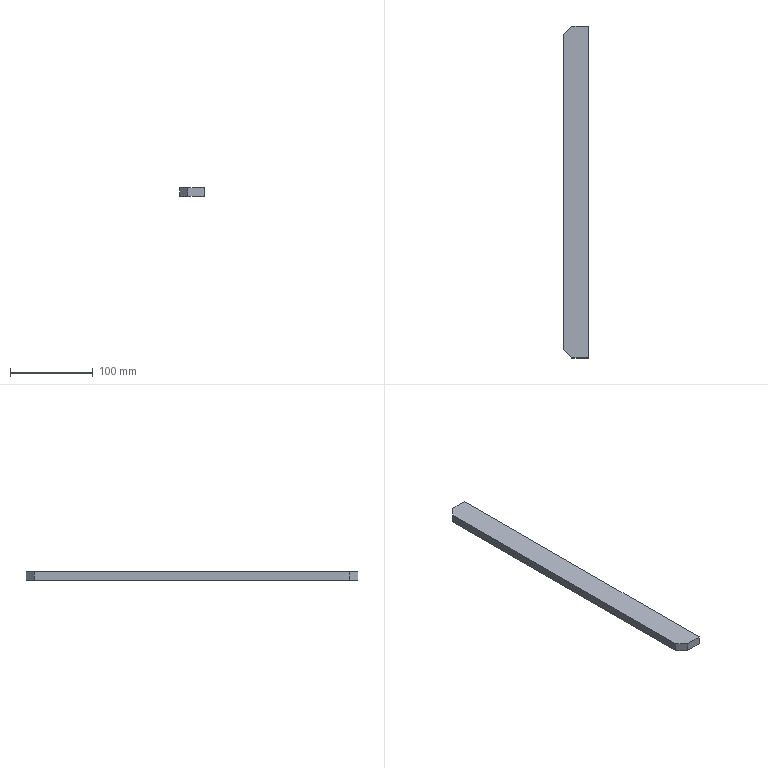Part | STEP file | DSJIN2 | 1 solid | 28 faces | box 30 x 400 x 10 mm | volume 118112 mm3 | cylinder 10 | cone 10 | plane 8 | commonest cylinder face diameters 4.2 x10
STEP:
#1=CARTESIAN_POINT('',(2.6,100.,6.1));
#2=VERTEX_POINT('',#1);
#3=CARTESIAN_POINT('',(2.6,100.,1.9));
#4=VERTEX_POINT('',#3);
#5=CARTESIAN_POINT('',(2.6,100.,4.));
#6=DIRECTION('',(1.,0.,0.));
#7=DIRECTION('',(0.,0.,-1.));
#8=AXIS2_PLACEMENT_3D('',#5,#6,#7);
#9=CIRCLE('',#8,2.1);
#10=EDGE_CURVE('',#2,#4,#9,.T.);
#11=ORIENTED_EDGE('',*,*,#10,.F.);
#12=CARTESIAN_POINT('',(15.,100.,6.1));
#13=VERTEX_POINT('',#12);
#14=CARTESIAN_POINT('',(15.,100.,6.1));
#15=DIRECTION('',(1.,0.,0.));
#16=VECTOR('',#15,1000.);
#17=LINE('',#14,#16);
#18=EDGE_CURVE('',#2,#13,#17,.T.);
#19=ORIENTED_EDGE('',*,*,#18,.T.);
#20=CARTESIAN_POINT('',(15.,100.,1.9));
#21=VERTEX_POINT('',#20);
#22=CARTESIAN_POINT('',(15.,100.,4.));
#23=DIRECTION('',(1.,0.,0.));
#24=DIRECTION('',(0.,0.,-1.));
#25=AXIS2_PLACEMENT_3D('',#22,#23,#24);
#26=CIRCLE('',#25,2.1);
#27=EDGE_CURVE('',#13,#21,#26,.T.);
#28=ORIENTED_EDGE('',*,*,#27,.T.);
#29=CARTESIAN_POINT('',(15.,100.,1.9));
#30=DIRECTION('',(1.,0.,0.));
#31=VECTOR('',#30,1000.);
#32=LINE('',#29,#31);
#33=EDGE_CURVE('',#4,#21,#32,.T.);
#34=ORIENTED_EDGE('',*,*,#33,.F.);
#35=EDGE_LOOP('',(#11,#19,#28,#34));
#36=FACE_OUTER_BOUND('',#35,.T.);
#37=CARTESIAN_POINT('',(15.,100.,4.));
#38=DIRECTION('',(1.,0.,0.));
#39=DIRECTION('',(0.,0.,-1.));
#40=AXIS2_PLACEMENT_3D('',#37,#38,#39);
#41=CYLINDRICAL_SURFACE('',#40,2.1);
#42=ADVANCED_FACE('',(#36),#41,.F.);
#43=CARTESIAN_POINT('',(1.338,100.,4.));
#44=VERTEX_POINT('',#43);
#45=CARTESIAN_POINT('',(2.6,100.,1.9));
#46=DIRECTION('',(0.515,0.,-0.8572));
#47=VECTOR('',#46,1000.);
#48=LINE('',#45,#47);
#49=EDGE_CURVE('',#44,#4,#48,.T.);
#50=ORIENTED_EDGE('',*,*,#49,.F.);
#51=CARTESIAN_POINT('',(2.6,100.,6.1));
#52=DIRECTION('',(0.515,0.,0.8572));
#53=VECTOR('',#52,1000.);
#54=LINE('',#51,#53);
#55=EDGE_CURVE('',#44,#2,#54,.T.);
#56=ORIENTED_EDGE('',*,*,#55,.T.);
#57=ORIENTED_EDGE('',*,*,#10,.T.);
#58=EDGE_LOOP('',(#50,#56,#57));
#59=FACE_OUTER_BOUND('',#58,.T.);
#60=CARTESIAN_POINT('',(2.6,100.,4.));
#61=DIRECTION('',(1.,0.,0.));
#62=DIRECTION('',(0.,0.,-1.));
#63=AXIS2_PLACEMENT_3D('',#60,#61,#62);
#64=CONICAL_SURFACE('',#63,2.1,1.03);
#65=ADVANCED_FACE('',(#59),#64,.F.);
#66=CARTESIAN_POINT('',(2.6,0.,6.1));
#67=VERTEX_POINT('',#66);
#68=CARTESIAN_POINT('',(2.6,0.,1.9));
#69=VERTEX_POINT('',#68);
#70=CARTESIAN_POINT('',(2.6,0.,4.));
#71=DIRECTION('',(1.,0.,0.));
#72=DIRECTION('',(0.,0.,-1.));
#73=AXIS2_PLACEMENT_3D('',#70,#71,#72);
#74=CIRCLE('',#73,2.1);
#75=EDGE_CURVE('',#67,#69,#74,.T.);
#76=ORIENTED_EDGE('',*,*,#75,.F.);
#77=CARTESIAN_POINT('',(15.,0.,6.1));
#78=VERTEX_POINT('',#77);
#79=CARTESIAN_POINT('',(15.,0.,6.1));
#80=DIRECTION('',(1.,0.,0.));
#81=VECTOR('',#80,1000.);
#82=LINE('',#79,#81);
#83=EDGE_CURVE('',#67,#78,#82,.T.);
#84=ORIENTED_EDGE('',*,*,#83,.T.);
#85=CARTESIAN_POINT('',(15.,0.,1.9));
#86=VERTEX_POINT('',#85);
#87=CARTESIAN_POINT('',(15.,0.,4.));
#88=DIRECTION('',(1.,0.,0.));
#89=DIRECTION('',(0.,0.,-1.));
#90=AXIS2_PLACEMENT_3D('',#87,#88,#89);
#91=CIRCLE('',#90,2.1);
#92=EDGE_CURVE('',#78,#86,#91,.T.);
#93=ORIENTED_EDGE('',*,*,#92,.T.);
#94=CARTESIAN_POINT('',(15.,0.,1.9));
#95=DIRECTION('',(1.,0.,0.));
#96=VECTOR('',#95,1000.);
#97=LINE('',#94,#96);
#98=EDGE_CURVE('',#69,#86,#97,.T.);
#99=ORIENTED_EDGE('',*,*,#98,.F.);
#100=EDGE_LOOP('',(#76,#84,#93,#99));
#101=FACE_OUTER_BOUND('',#100,.T.);
#102=CARTESIAN_POINT('',(15.,0.,4.));
#103=DIRECTION('',(1.,0.,0.));
#104=DIRECTION('',(0.,0.,-1.));
#105=AXIS2_PLACEMENT_3D('',#102,#103,#104);
#106=CYLINDRICAL_SURFACE('',#105,2.1);
#107=ADVANCED_FACE('',(#101),#106,.F.);
#108=CARTESIAN_POINT('',(1.338,0.,4.));
#109=VERTEX_POINT('',#108);
#110=CARTESIAN_POINT('',(2.6,0.,1.9));
#111=DIRECTION('',(0.515,0.,-0.8572));
#112=VECTOR('',#111,1000.);
#113=LINE('',#110,#112);
#114=EDGE_CURVE('',#109,#69,#113,.T.);
#115=ORIENTED_EDGE('',*,*,#114,.F.);
#116=CARTESIAN_POINT('',(2.6,0.,6.1));
#117=DIRECTION('',(0.515,0.,0.8572));
#118=VECTOR('',#117,1000.);
#119=LINE('',#116,#118);
#120=EDGE_CURVE('',#109,#67,#119,.T.);
#121=ORIENTED_EDGE('',*,*,#120,.T.);
#122=ORIENTED_EDGE('',*,*,#75,.T.);
#123=EDGE_LOOP('',(#115,#121,#122));
#124=FACE_OUTER_BOUND('',#123,.T.);
#125=CARTESIAN_POINT('',(2.6,0.,4.));
#126=DIRECTION('',(1.,0.,0.));
#127=DIRECTION('',(0.,0.,-1.));
#128=AXIS2_PLACEMENT_3D('',#125,#126,#127);
#129=CONICAL_SURFACE('',#128,2.1,1.03);
#130=ADVANCED_FACE('',(#124),#129,.F.);
#131=CARTESIAN_POINT('',(2.6,-100.,6.1));
#132=VERTEX_POINT('',#131);
#133=CARTESIAN_POINT('',(2.6,-100.,1.9));
#134=VERTEX_POINT('',#133);
#135=CARTESIAN_POINT('',(2.6,-100.,4.));
#136=DIRECTION('',(1.,0.,0.));
#137=DIRECTION('',(0.,0.,-1.));
#138=AXIS2_PLACEMENT_3D('',#135,#136,#137);
#139=CIRCLE('',#138,2.1);
#140=EDGE_CURVE('',#132,#134,#139,.T.);
#141=ORIENTED_EDGE('',*,*,#140,.F.);
#142=CARTESIAN_POINT('',(15.,-100.,6.1));
#143=VERTEX_POINT('',#142);
#144=CARTESIAN_POINT('',(15.,-100.,6.1));
#145=DIRECTION('',(1.,0.,0.));
#146=VECTOR('',#145,1000.);
#147=LINE('',#144,#146);
#148=EDGE_CURVE('',#132,#143,#147,.T.);
#149=ORIENTED_EDGE('',*,*,#148,.T.);
#150=CARTESIAN_POINT('',(15.,-100.,1.9));
#151=VERTEX_POINT('',#150);
#152=CARTESIAN_POINT('',(15.,-100.,4.));
#153=DIRECTION('',(1.,0.,0.));
#154=DIRECTION('',(0.,0.,-1.));
#155=AXIS2_PLACEMENT_3D('',#152,#153,#154);
#156=CIRCLE('',#155,2.1);
#157=EDGE_CURVE('',#143,#151,#156,.T.);
#158=ORIENTED_EDGE('',*,*,#157,.T.);
#159=CARTESIAN_POINT('',(15.,-100.,1.9));
#160=DIRECTION('',(1.,0.,0.));
#161=VECTOR('',#160,1000.);
#162=LINE('',#159,#161);
#163=EDGE_CURVE('',#134,#151,#162,.T.);
#164=ORIENTED_EDGE('',*,*,#163,.F.);
#165=EDGE_LOOP('',(#141,#149,#158,#164));
#166=FACE_OUTER_BOUND('',#165,.T.);
#167=CARTESIAN_POINT('',(15.,-100.,4.));
#168=DIRECTION('',(1.,0.,0.));
#169=DIRECTION('',(0.,0.,-1.));
#170=AXIS2_PLACEMENT_3D('',#167,#168,#169);
#171=CYLINDRICAL_SURFACE('',#170,2.1);
#172=ADVANCED_FACE('',(#166),#171,.F.);
#173=CARTESIAN_POINT('',(1.338,-100.,4.));
#174=VERTEX_POINT('',#173);
#175=CARTESIAN_POINT('',(2.6,-100.,1.9));
#176=DIRECTION('',(0.515,0.,-0.8572));
#177=VECTOR('',#176,1000.);
#178=LINE('',#175,#177);
#179=EDGE_CURVE('',#174,#134,#178,.T.);
#180=ORIENTED_EDGE('',*,*,#179,.F.);
#181=CARTESIAN_POINT('',(2.6,-100.,6.1));
#182=DIRECTION('',(0.515,0.,0.8572));
#183=VECTOR('',#182,1000.);
#184=LINE('',#181,#183);
#185=EDGE_CURVE('',#174,#132,#184,.T.);
#186=ORIENTED_EDGE('',*,*,#185,.T.);
#187=ORIENTED_EDGE('',*,*,#140,.T.);
#188=EDGE_LOOP('',(#180,#186,#187));
#189=FACE_OUTER_BOUND('',#188,.T.);
#190=CARTESIAN_POINT('',(2.6,-100.,4.));
#191=DIRECTION('',(1.,0.,0.));
#192=DIRECTION('',(0.,0.,-1.));
#193=AXIS2_PLACEMENT_3D('',#190,#191,#192);
#194=CONICAL_SURFACE('',#193,2.1,1.03);
#195=ADVANCED_FACE('',(#189),#194,.F.);
#196=CARTESIAN_POINT('',(2.6,190.,6.1));
#197=VERTEX_POINT('',#196);
#198=CARTESIAN_POINT('',(2.6,190.,1.9));
#199=VERTEX_POINT('',#198);
#200=CARTESIAN_POINT('',(2.6,190.,4.));
#201=DIRECTION('',(1.,0.,0.));
#202=DIRECTION('',(0.,0.,-1.));
#203=AXIS2_PLACEMENT_3D('',#200,#201,#202);
#204=CIRCLE('',#203,2.1);
#205=EDGE_CURVE('',#197,#199,#204,.T.);
#206=ORIENTED_EDGE('',*,*,#205,.F.);
#207=CARTESIAN_POINT('',(15.,190.,6.1));
#208=VERTEX_POINT('',#207);
#209=CARTESIAN_POINT('',(15.,190.,6.1));
#210=DIRECTION('',(1.,0.,0.));
#211=VECTOR('',#210,1000.);
#212=LINE('',#209,#211);
#213=EDGE_CURVE('',#197,#208,#212,.T.);
#214=ORIENTED_EDGE('',*,*,#213,.T.);
#215=CARTESIAN_POINT('',(15.,190.,1.9));
#216=VERTEX_POINT('',#215);
#217=CARTESIAN_POINT('',(15.,190.,4.));
#218=DIRECTION('',(1.,0.,0.));
#219=DIRECTION('',(0.,0.,-1.));
#220=AXIS2_PLACEMENT_3D('',#217,#218,#219);
#221=CIRCLE('',#220,2.1);
#222=EDGE_CURVE('',#208,#216,#221,.T.);
#223=ORIENTED_EDGE('',*,*,#222,.T.);
#224=CARTESIAN_POINT('',(15.,190.,1.9));
#225=DIRECTION('',(1.,0.,0.));
#226=VECTOR('',#225,1000.);
#227=LINE('',#224,#226);
#228=EDGE_CURVE('',#199,#216,#227,.T.);
#229=ORIENTED_EDGE('',*,*,#228,.F.);
#230=EDGE_LOOP('',(#206,#214,#223,#229));
#231=FACE_OUTER_BOUND('',#230,.T.);
#232=CARTESIAN_POINT('',(15.,190.,4.));
#233=DIRECTION('',(1.,0.,0.));
#234=DIRECTION('',(0.,0.,-1.));
#235=AXIS2_PLACEMENT_3D('',#232,#233,#234);
#236=CYLINDRICAL_SURFACE('',#235,2.1);
#237=ADVANCED_FACE('',(#231),#236,.F.);
#238=CARTESIAN_POINT('',(1.338,190.,4.));
#239=VERTEX_POINT('',#238);
#240=CARTESIAN_POINT('',(2.6,190.,1.9));
#241=DIRECTION('',(0.515,0.,-0.8572));
#242=VECTOR('',#241,1000.);
#243=LINE('',#240,#242);
#244=EDGE_CURVE('',#239,#199,#243,.T.);
#245=ORIENTED_EDGE('',*,*,#244,.F.);
#246=CARTESIAN_POINT('',(2.6,190.,6.1));
#247=DIRECTION('',(0.515,0.,0.8572));
#248=VECTOR('',#247,1000.);
#249=LINE('',#246,#248);
#250=EDGE_CURVE('',#239,#197,#249,.T.);
#251=ORIENTED_EDGE('',*,*,#250,.T.);
#252=ORIENTED_EDGE('',*,*,#205,.T.);
#253=EDGE_LOOP('',(#245,#251,#252));
#254=FACE_OUTER_BOUND('',#253,.T.);
#255=CARTESIAN_POINT('',(2.6,190.,4.));
#256=DIRECTION('',(1.,0.,0.));
#257=DIRECTION('',(0.,0.,-1.));
#258=AXIS2_PLACEMENT_3D('',#255,#256,#257);
#259=CONICAL_SURFACE('',#258,2.1,1.03);
#260=ADVANCED_FACE('',(#254),#259,.F.);
#261=CARTESIAN_POINT('',(2.6,-190.,6.1));
#262=VERTEX_POINT('',#261);
#263=CARTESIAN_POINT('',(2.6,-190.,1.9));
#264=VERTEX_POINT('',#263);
#265=CARTESIAN_POINT('',(2.6,-190.,4.));
#266=DIRECTION('',(1.,0.,0.));
#267=DIRECTION('',(0.,0.,-1.));
#268=AXIS2_PLACEMENT_3D('',#265,#266,#267);
#269=CIRCLE('',#268,2.1);
#270=EDGE_CURVE('',#262,#264,#269,.T.);
#271=ORIENTED_EDGE('',*,*,#270,.F.);
#272=CARTESIAN_POINT('',(15.,-190.,6.1));
#273=VERTEX_POINT('',#272);
#274=CARTESIAN_POINT('',(15.,-190.,6.1));
#275=DIRECTION('',(1.,0.,0.));
#276=VECTOR('',#275,1000.);
#277=LINE('',#274,#276);
#278=EDGE_CURVE('',#262,#273,#277,.T.);
#279=ORIENTED_EDGE('',*,*,#278,.T.);
#280=CARTESIAN_POINT('',(15.,-190.,1.9));
#281=VERTEX_POINT('',#280);
#282=CARTESIAN_POINT('',(15.,-190.,4.));
#283=DIRECTION('',(1.,0.,0.));
#284=DIRECTION('',(0.,0.,-1.));
#285=AXIS2_PLACEMENT_3D('',#282,#283,#284);
#286=CIRCLE('',#285,2.1);
#287=EDGE_CURVE('',#273,#281,#286,.T.);
#288=ORIENTED_EDGE('',*,*,#287,.T.);
#289=CARTESIAN_POINT('',(15.,-190.,1.9));
#290=DIRECTION('',(1.,0.,0.));
#291=VECTOR('',#290,1000.);
#292=LINE('',#289,#291);
#293=EDGE_CURVE('',#264,#281,#292,.T.);
#294=ORIENTED_EDGE('',*,*,#293,.F.);
#295=EDGE_LOOP('',(#271,#279,#288,#294));
#296=FACE_OUTER_BOUND('',#295,.T.);
#297=CARTESIAN_POINT('',(15.,-190.,4.));
#298=DIRECTION('',(1.,0.,0.));
#299=DIRECTION('',(0.,0.,-1.));
#300=AXIS2_PLACEMENT_3D('',#297,#298,#299);
#301=CYLINDRICAL_SURFACE('',#300,2.1);
#302=ADVANCED_FACE('',(#296),#301,.F.);
#303=CARTESIAN_POINT('',(1.338,-190.,4.));
#304=VERTEX_POINT('',#303);
#305=CARTESIAN_POINT('',(2.6,-190.,1.9));
#306=DIRECTION('',(0.515,0.,-0.8572));
#307=VECTOR('',#306,1000.);
#308=LINE('',#305,#307);
#309=EDGE_CURVE('',#304,#264,#308,.T.);
#310=ORIENTED_EDGE('',*,*,#309,.F.);
#311=CARTESIAN_POINT('',(2.6,-190.,6.1));
#312=DIRECTION('',(0.515,0.,0.8572));
#313=VECTOR('',#312,1000.);
#314=LINE('',#311,#313);
#315=EDGE_CURVE('',#304,#262,#314,.T.);
#316=ORIENTED_EDGE('',*,*,#315,.T.);
#317=ORIENTED_EDGE('',*,*,#270,.T.);
#318=EDGE_LOOP('',(#310,#316,#317));
#319=FACE_OUTER_BOUND('',#318,.T.);
#320=CARTESIAN_POINT('',(2.6,-190.,4.));
#321=DIRECTION('',(1.,0.,0.));
#322=DIRECTION('',(0.,0.,-1.));
#323=AXIS2_PLACEMENT_3D('',#320,#321,#322);
#324=CONICAL_SURFACE('',#323,2.1,1.03);
#325=ADVANCED_FACE('',(#319),#324,.F.);
#326=CARTESIAN_POINT('',(15.,100.,4.));
#327=DIRECTION('',(1.,0.,0.));
#328=DIRECTION('',(0.,0.,-1.));
#329=AXIS2_PLACEMENT_3D('',#326,#327,#328);
#330=CIRCLE('',#329,2.1);
#331=EDGE_CURVE('',#21,#13,#330,.T.);
#332=ORIENTED_EDGE('',*,*,#331,.F.);
#333=ORIENTED_EDGE('',*,*,#27,.F.);
#334=EDGE_LOOP('',(#332,#333));
#335=FACE_BOUND('',#334,.T.);
#336=CARTESIAN_POINT('',(15.,0.,4.));
#337=DIRECTION('',(1.,0.,0.));
#338=DIRECTION('',(0.,0.,-1.));
#339=AXIS2_PLACEMENT_3D('',#336,#337,#338);
#340=CIRCLE('',#339,2.1);
#341=EDGE_CURVE('',#86,#78,#340,.T.);
#342=ORIENTED_EDGE('',*,*,#341,.F.);
#343=ORIENTED_EDGE('',*,*,#92,.F.);
#344=EDGE_LOOP('',(#342,#343));
#345=FACE_BOUND('',#344,.T.);
#346=CARTESIAN_POINT('',(15.,-100.,4.));
#347=DIRECTION('',(1.,0.,0.));
#348=DIRECTION('',(0.,0.,-1.));
#349=AXIS2_PLACEMENT_3D('',#346,#347,#348);
#350=CIRCLE('',#349,2.1);
#351=EDGE_CURVE('',#151,#143,#350,.T.);
#352=ORIENTED_EDGE('',*,*,#351,.F.);
#353=ORIENTED_EDGE('',*,*,#157,.F.);
#354=EDGE_LOOP('',(#352,#353));
#355=FACE_BOUND('',#354,.T.);
#356=CARTESIAN_POINT('',(15.,190.,4.));
#357=DIRECTION('',(1.,0.,0.));
#358=DIRECTION('',(0.,0.,-1.));
#359=AXIS2_PLACEMENT_3D('',#356,#357,#358);
#360=CIRCLE('',#359,2.1);
#361=EDGE_CURVE('',#216,#208,#360,.T.);
#362=ORIENTED_EDGE('',*,*,#361,.F.);
#363=ORIENTED_EDGE('',*,*,#222,.F.);
#364=EDGE_LOOP('',(#362,#363));
#365=FACE_BOUND('',#364,.T.);
#366=CARTESIAN_POINT('',(15.,-190.,4.));
#367=DIRECTION('',(1.,0.,0.));
#368=DIRECTION('',(0.,0.,-1.));
#369=AXIS2_PLACEMENT_3D('',#366,#367,#368);
#370=CIRCLE('',#369,2.1);
#371=EDGE_CURVE('',#281,#273,#370,.T.);
#372=ORIENTED_EDGE('',*,*,#371,.F.);
#373=ORIENTED_EDGE('',*,*,#287,.F.);
#374=EDGE_LOOP('',(#372,#373));
#375=FACE_BOUND('',#374,.T.);
#376=CARTESIAN_POINT('',(15.,-200.,0.));
#377=VERTEX_POINT('',#376);
#378=CARTESIAN_POINT('',(15.,200.,0.));
#379=VERTEX_POINT('',#378);
#380=CARTESIAN_POINT('',(15.,-200.,0.));
#381=DIRECTION('',(0.,1.,0.));
#382=VECTOR('',#381,1000.);
#383=LINE('',#380,#382);
#384=EDGE_CURVE('',#377,#379,#383,.T.);
#385=ORIENTED_EDGE('',*,*,#384,.T.);
#386=CARTESIAN_POINT('',(15.,200.,10.));
#387=VERTEX_POINT('',#386);
#388=CARTESIAN_POINT('',(15.,200.,10.));
#389=DIRECTION('',(0.,0.,-1.));
#390=VECTOR('',#389,1000.);
#391=LINE('',#388,#390);
#392=EDGE_CURVE('',#387,#379,#391,.T.);
#393=ORIENTED_EDGE('',*,*,#392,.F.);
#394=CARTESIAN_POINT('',(15.,-200.,10.));
#395=VERTEX_POINT('',#394);
#396=CARTESIAN_POINT('',(15.,-200.,10.));
#397=DIRECTION('',(0.,1.,0.));
#398=VECTOR('',#397,1000.);
#399=LINE('',#396,#398);
#400=EDGE_CURVE('',#395,#387,#399,.T.);
#401=ORIENTED_EDGE('',*,*,#400,.F.);
#402=CARTESIAN_POINT('',(15.,-200.,10.));
#403=DIRECTION('',(0.,0.,-1.));
#404=VECTOR('',#403,1000.);
#405=LINE('',#402,#404);
#406=EDGE_CURVE('',#395,#377,#405,.T.);
#407=ORIENTED_EDGE('',*,*,#406,.T.);
#408=EDGE_LOOP('',(#385,#393,#401,#407));
#409=FACE_OUTER_BOUND('',#408,.T.);
#410=CARTESIAN_POINT('',(15.,-200.,10.));
#411=DIRECTION('',(-1.,0.,0.));
#412=DIRECTION('',(0.,0.,1.));
#413=AXIS2_PLACEMENT_3D('',#410,#411,#412);
#414=PLANE('',#413);
#415=ADVANCED_FACE('',(#335,#345,#355,#365,#375,#409),#414,.F.);
#416=CARTESIAN_POINT('',(-5.,200.,0.));
#417=VERTEX_POINT('',#416);
#418=CARTESIAN_POINT('',(-15.,200.,0.));
#419=DIRECTION('',(-1.,0.,0.));
#420=VECTOR('',#419,1000.);
#421=LINE('',#418,#420);
#422=EDGE_CURVE('',#379,#417,#421,.T.);
#423=ORIENTED_EDGE('',*,*,#422,.T.);
#424=CARTESIAN_POINT('',(-5.,200.,10.));
#425=VERTEX_POINT('',#424);
#426=CARTESIAN_POINT('',(-5.,200.,10.));
#427=DIRECTION('',(0.,0.,1.));
#428=VECTOR('',#427,1000.);
#429=LINE('',#426,#428);
#430=EDGE_CURVE('',#417,#425,#429,.T.);
#431=ORIENTED_EDGE('',*,*,#430,.T.);
#432=CARTESIAN_POINT('',(-15.,200.,10.));
#433=DIRECTION('',(-1.,0.,0.));
#434=VECTOR('',#433,1000.);
#435=LINE('',#432,#434);
#436=EDGE_CURVE('',#387,#425,#435,.T.);
#437=ORIENTED_EDGE('',*,*,#436,.F.);
#438=ORIENTED_EDGE('',*,*,#392,.T.);
#439=EDGE_LOOP('',(#423,#431,#437,#438));
#440=FACE_OUTER_BOUND('',#439,.T.);
#441=CARTESIAN_POINT('',(-15.,200.,10.));
#442=DIRECTION('',(0.,-1.,0.));
#443=DIRECTION('',(0.,0.,-1.));
#444=AXIS2_PLACEMENT_3D('',#441,#442,#443);
#445=PLANE('',#444);
#446=ADVANCED_FACE('',(#440),#445,.F.);
#447=CARTESIAN_POINT('',(-15.,190.,10.));
#448=VERTEX_POINT('',#447);
#449=CARTESIAN_POINT('',(-15.,-190.,10.));
#450=VERTEX_POINT('',#449);
#451=CARTESIAN_POINT('',(-15.,-200.,10.));
#452=DIRECTION('',(0.,-1.,0.));
#453=VECTOR('',#452,1000.);
#454=LINE('',#451,#453);
#455=EDGE_CURVE('',#448,#450,#454,.T.);
#456=ORIENTED_EDGE('',*,*,#455,.F.);
#457=CARTESIAN_POINT('',(-15.,190.,0.));
#458=VERTEX_POINT('',#457);
#459=CARTESIAN_POINT('',(-15.,190.,10.));
#460=DIRECTION('',(0.,0.,-1.));
#461=VECTOR('',#460,1000.);
#462=LINE('',#459,#461);
#463=EDGE_CURVE('',#448,#458,#462,.T.);
#464=ORIENTED_EDGE('',*,*,#463,.T.);
#465=CARTESIAN_POINT('',(-15.,-190.,0.));
#466=VERTEX_POINT('',#465);
#467=CARTESIAN_POINT('',(-15.,-200.,0.));
#468=DIRECTION('',(0.,-1.,0.));
#469=VECTOR('',#468,1000.);
#470=LINE('',#467,#469);
#471=EDGE_CURVE('',#458,#466,#470,.T.);
#472=ORIENTED_EDGE('',*,*,#471,.T.);
#473=CARTESIAN_POINT('',(-15.,-190.,10.));
#474=DIRECTION('',(0.,0.,1.));
#475=VECTOR('',#474,1000.);
#476=LINE('',#473,#475);
#477=EDGE_CURVE('',#466,#450,#476,.T.);
#478=ORIENTED_EDGE('',*,*,#477,.T.);
#479=EDGE_LOOP('',(#456,#464,#472,#478));
#480=FACE_OUTER_BOUND('',#479,.T.);
#481=CARTESIAN_POINT('',(-15.,-200.,10.));
#482=DIRECTION('',(1.,0.,0.));
#483=DIRECTION('',(0.,0.,-1.));
#484=AXIS2_PLACEMENT_3D('',#481,#482,#483);
#485=PLANE('',#484);
#486=ADVANCED_FACE('',(#480),#485,.F.);
#487=CARTESIAN_POINT('',(-5.,-200.,10.));
#488=VERTEX_POINT('',#487);
#489=CARTESIAN_POINT('',(-15.,-200.,10.));
#490=DIRECTION('',(1.,0.,0.));
#491=VECTOR('',#490,1000.);
#492=LINE('',#489,#491);
#493=EDGE_CURVE('',#488,#395,#492,.T.);
#494=ORIENTED_EDGE('',*,*,#493,.F.);
#495=CARTESIAN_POINT('',(-5.,-200.,0.));
#496=VERTEX_POINT('',#495);
#497=CARTESIAN_POINT('',(-5.,-200.,10.));
#498=DIRECTION('',(0.,0.,-1.));
#499=VECTOR('',#498,1000.);
#500=LINE('',#497,#499);
#501=EDGE_CURVE('',#488,#496,#500,.T.);
#502=ORIENTED_EDGE('',*,*,#501,.T.);
#503=CARTESIAN_POINT('',(-15.,-200.,0.));
#504=DIRECTION('',(1.,0.,0.));
#505=VECTOR('',#504,1000.);
#506=LINE('',#503,#505);
#507=EDGE_CURVE('',#496,#377,#506,.T.);
#508=ORIENTED_EDGE('',*,*,#507,.T.);
#509=ORIENTED_EDGE('',*,*,#406,.F.);
#510=EDGE_LOOP('',(#494,#502,#508,#509));
#511=FACE_OUTER_BOUND('',#510,.T.);
#512=CARTESIAN_POINT('',(-15.,-200.,10.));
#513=DIRECTION('',(0.,1.,0.));
#514=DIRECTION('',(0.,0.,1.));
#515=AXIS2_PLACEMENT_3D('',#512,#513,#514);
#516=PLANE('',#515);
#517=ADVANCED_FACE('',(#511),#516,.F.);
#518=ORIENTED_EDGE('',*,*,#436,.T.);
#519=CARTESIAN_POINT('',(-15.,190.,10.));
#520=DIRECTION('',(-0.7071,-0.7071,0.));
#521=VECTOR('',#520,1000.);
#522=LINE('',#519,#521);
#523=EDGE_CURVE('',#425,#448,#522,.T.);
#524=ORIENTED_EDGE('',*,*,#523,.T.);
#525=ORIENTED_EDGE('',*,*,#455,.T.);
#526=CARTESIAN_POINT('',(-5.,-200.,10.));
#527=DIRECTION('',(0.7071,-0.7071,0.));
#528=VECTOR('',#527,1000.);
#529=LINE('',#526,#528);
#530=EDGE_CURVE('',#450,#488,#529,.T.);
#531=ORIENTED_EDGE('',*,*,#530,.T.);
#532=ORIENTED_EDGE('',*,*,#493,.T.);
#533=ORIENTED_EDGE('',*,*,#400,.T.);
#534=EDGE_LOOP('',(#518,#524,#525,#531,#532,#533));
#535=FACE_OUTER_BOUND('',#534,.T.);
#536=CARTESIAN_POINT('',(0.,0.,10.));
#537=DIRECTION('',(0.,0.,-1.));
#538=DIRECTION('',(-1.,0.,0.));
#539=AXIS2_PLACEMENT_3D('',#536,#537,#538);
#540=PLANE('',#539);
#541=ADVANCED_FACE('',(#535),#540,.F.);
#542=ORIENTED_EDGE('',*,*,#471,.F.);
#543=CARTESIAN_POINT('',(-102.5,102.5,0.));
#544=DIRECTION('',(0.7071,0.7071,0.));
#545=VECTOR('',#544,1000.);
#546=LINE('',#543,#545);
#547=EDGE_CURVE('',#458,#417,#546,.T.);
#548=ORIENTED_EDGE('',*,*,#547,.T.);
#549=ORIENTED_EDGE('',*,*,#422,.F.);
#550=ORIENTED_EDGE('',*,*,#384,.F.);
#551=ORIENTED_EDGE('',*,*,#507,.F.);
#552=CARTESIAN_POINT('',(-102.5,-102.5,0.));
#553=DIRECTION('',(-0.7071,0.7071,0.));
#554=VECTOR('',#553,1000.);
#555=LINE('',#552,#554);
#556=EDGE_CURVE('',#496,#466,#555,.T.);
#557=ORIENTED_EDGE('',*,*,#556,.T.);
#558=EDGE_LOOP('',(#542,#548,#549,#550,#551,#557));
#559=FACE_OUTER_BOUND('',#558,.T.);
#560=CARTESIAN_POINT('',(0.,0.,0.));
#561=DIRECTION('',(0.,0.,-1.));
#562=DIRECTION('',(-1.,0.,0.));
#563=AXIS2_PLACEMENT_3D('',#560,#561,#562);
#564=PLANE('',#563);
#565=ADVANCED_FACE('',(#559),#564,.T.);
#566=ORIENTED_EDGE('',*,*,#315,.F.);
#567=ORIENTED_EDGE('',*,*,#309,.T.);
#568=CARTESIAN_POINT('',(2.6,-190.,4.));
#569=DIRECTION('',(1.,0.,0.));
#570=DIRECTION('',(0.,0.,-1.));
#571=AXIS2_PLACEMENT_3D('',#568,#569,#570);
#572=CIRCLE('',#571,2.1);
#573=EDGE_CURVE('',#264,#262,#572,.T.);
#574=ORIENTED_EDGE('',*,*,#573,.T.);
#575=EDGE_LOOP('',(#566,#567,#574));
#576=FACE_OUTER_BOUND('',#575,.T.);
#577=CARTESIAN_POINT('',(2.6,-190.,4.));
#578=DIRECTION('',(1.,0.,0.));
#579=DIRECTION('',(0.,0.,-1.));
#580=AXIS2_PLACEMENT_3D('',#577,#578,#579);
#581=CONICAL_SURFACE('',#580,2.1,1.03);
#582=ADVANCED_FACE('',(#576),#581,.F.);
#583=ORIENTED_EDGE('',*,*,#278,.F.);
#584=ORIENTED_EDGE('',*,*,#573,.F.);
#585=ORIENTED_EDGE('',*,*,#293,.T.);
#586=ORIENTED_EDGE('',*,*,#371,.T.);
#587=EDGE_LOOP('',(#583,#584,#585,#586));
#588=FACE_OUTER_BOUND('',#587,.T.);
#589=CARTESIAN_POINT('',(15.,-190.,4.));
#590=DIRECTION('',(1.,0.,0.));
#591=DIRECTION('',(0.,0.,-1.));
#592=AXIS2_PLACEMENT_3D('',#589,#590,#591);
#593=CYLINDRICAL_SURFACE('',#592,2.1);
#594=ADVANCED_FACE('',(#588),#593,.F.);
#595=ORIENTED_EDGE('',*,*,#250,.F.);
#596=ORIENTED_EDGE('',*,*,#244,.T.);
#597=CARTESIAN_POINT('',(2.6,190.,4.));
#598=DIRECTION('',(1.,0.,0.));
#599=DIRECTION('',(0.,0.,-1.));
#600=AXIS2_PLACEMENT_3D('',#597,#598,#599);
#601=CIRCLE('',#600,2.1);
#602=EDGE_CURVE('',#199,#197,#601,.T.);
#603=ORIENTED_EDGE('',*,*,#602,.T.);
#604=EDGE_LOOP('',(#595,#596,#603));
#605=FACE_OUTER_BOUND('',#604,.T.);
#606=CARTESIAN_POINT('',(2.6,190.,4.));
#607=DIRECTION('',(1.,0.,0.));
#608=DIRECTION('',(0.,0.,-1.));
#609=AXIS2_PLACEMENT_3D('',#606,#607,#608);
#610=CONICAL_SURFACE('',#609,2.1,1.03);
#611=ADVANCED_FACE('',(#605),#610,.F.);
#612=ORIENTED_EDGE('',*,*,#213,.F.);
#613=ORIENTED_EDGE('',*,*,#602,.F.);
#614=ORIENTED_EDGE('',*,*,#228,.T.);
#615=ORIENTED_EDGE('',*,*,#361,.T.);
#616=EDGE_LOOP('',(#612,#613,#614,#615));
#617=FACE_OUTER_BOUND('',#616,.T.);
#618=CARTESIAN_POINT('',(15.,190.,4.));
#619=DIRECTION('',(1.,0.,0.));
#620=DIRECTION('',(0.,0.,-1.));
#621=AXIS2_PLACEMENT_3D('',#618,#619,#620);
#622=CYLINDRICAL_SURFACE('',#621,2.1);
#623=ADVANCED_FACE('',(#617),#622,.F.);
#624=ORIENTED_EDGE('',*,*,#185,.F.);
#625=ORIENTED_EDGE('',*,*,#179,.T.);
#626=CARTESIAN_POINT('',(2.6,-100.,4.));
#627=DIRECTION('',(1.,0.,0.));
#628=DIRECTION('',(0.,0.,-1.));
#629=AXIS2_PLACEMENT_3D('',#626,#627,#628);
#630=CIRCLE('',#629,2.1);
#631=EDGE_CURVE('',#134,#132,#630,.T.);
#632=ORIENTED_EDGE('',*,*,#631,.T.);
#633=EDGE_LOOP('',(#624,#625,#632));
#634=FACE_OUTER_BOUND('',#633,.T.);
#635=CARTESIAN_POINT('',(2.6,-100.,4.));
#636=DIRECTION('',(1.,0.,0.));
#637=DIRECTION('',(0.,0.,-1.));
#638=AXIS2_PLACEMENT_3D('',#635,#636,#637);
#639=CONICAL_SURFACE('',#638,2.1,1.03);
#640=ADVANCED_FACE('',(#634),#639,.F.);
#641=ORIENTED_EDGE('',*,*,#148,.F.);
#642=ORIENTED_EDGE('',*,*,#631,.F.);
#643=ORIENTED_EDGE('',*,*,#163,.T.);
#644=ORIENTED_EDGE('',*,*,#351,.T.);
#645=EDGE_LOOP('',(#641,#642,#643,#644));
#646=FACE_OUTER_BOUND('',#645,.T.);
#647=CARTESIAN_POINT('',(15.,-100.,4.));
#648=DIRECTION('',(1.,0.,0.));
#649=DIRECTION('',(0.,0.,-1.));
#650=AXIS2_PLACEMENT_3D('',#647,#648,#649);
#651=CYLINDRICAL_SURFACE('',#650,2.1);
#652=ADVANCED_FACE('',(#646),#651,.F.);
#653=ORIENTED_EDGE('',*,*,#120,.F.);
#654=ORIENTED_EDGE('',*,*,#114,.T.);
#655=CARTESIAN_POINT('',(2.6,0.,4.));
#656=DIRECTION('',(1.,0.,0.));
#657=DIRECTION('',(0.,0.,-1.));
#658=AXIS2_PLACEMENT_3D('',#655,#656,#657);
#659=CIRCLE('',#658,2.1);
#660=EDGE_CURVE('',#69,#67,#659,.T.);
#661=ORIENTED_EDGE('',*,*,#660,.T.);
#662=EDGE_LOOP('',(#653,#654,#661));
#663=FACE_OUTER_BOUND('',#662,.T.);
#664=CARTESIAN_POINT('',(2.6,0.,4.));
#665=DIRECTION('',(1.,0.,0.));
#666=DIRECTION('',(0.,0.,-1.));
#667=AXIS2_PLACEMENT_3D('',#664,#665,#666);
#668=CONICAL_SURFACE('',#667,2.1,1.03);
#669=ADVANCED_FACE('',(#663),#668,.F.);
#670=ORIENTED_EDGE('',*,*,#83,.F.);
#671=ORIENTED_EDGE('',*,*,#660,.F.);
#672=ORIENTED_EDGE('',*,*,#98,.T.);
#673=ORIENTED_EDGE('',*,*,#341,.T.);
#674=EDGE_LOOP('',(#670,#671,#672,#673));
#675=FACE_OUTER_BOUND('',#674,.T.);
#676=CARTESIAN_POINT('',(15.,0.,4.));
#677=DIRECTION('',(1.,0.,0.));
#678=DIRECTION('',(0.,0.,-1.));
#679=AXIS2_PLACEMENT_3D('',#676,#677,#678);
#680=CYLINDRICAL_SURFACE('',#679,2.1);
#681=ADVANCED_FACE('',(#675),#680,.F.);
#682=ORIENTED_EDGE('',*,*,#55,.F.);
#683=ORIENTED_EDGE('',*,*,#49,.T.);
#684=CARTESIAN_POINT('',(2.6,100.,4.));
#685=DIRECTION('',(1.,0.,0.));
#686=DIRECTION('',(0.,0.,-1.));
#687=AXIS2_PLACEMENT_3D('',#684,#685,#686);
#688=CIRCLE('',#687,2.1);
#689=EDGE_CURVE('',#4,#2,#688,.T.);
#690=ORIENTED_EDGE('',*,*,#689,.T.);
#691=EDGE_LOOP('',(#682,#683,#690));
#692=FACE_OUTER_BOUND('',#691,.T.);
#693=CARTESIAN_POINT('',(2.6,100.,4.));
#694=DIRECTION('',(1.,0.,0.));
#695=DIRECTION('',(0.,0.,-1.));
#696=AXIS2_PLACEMENT_3D('',#693,#694,#695);
#697=CONICAL_SURFACE('',#696,2.1,1.03);
#698=ADVANCED_FACE('',(#692),#697,.F.);
#699=ORIENTED_EDGE('',*,*,#18,.F.);
#700=ORIENTED_EDGE('',*,*,#689,.F.);
#701=ORIENTED_EDGE('',*,*,#33,.T.);
#702=ORIENTED_EDGE('',*,*,#331,.T.);
#703=EDGE_LOOP('',(#699,#700,#701,#702));
#704=FACE_OUTER_BOUND('',#703,.T.);
#705=CARTESIAN_POINT('',(15.,100.,4.));
#706=DIRECTION('',(1.,0.,0.));
#707=DIRECTION('',(0.,0.,-1.));
#708=AXIS2_PLACEMENT_3D('',#705,#706,#707);
#709=CYLINDRICAL_SURFACE('',#708,2.1);
#710=ADVANCED_FACE('',(#704),#709,.F.);
#711=ORIENTED_EDGE('',*,*,#523,.F.);
#712=ORIENTED_EDGE('',*,*,#430,.F.);
#713=ORIENTED_EDGE('',*,*,#547,.F.);
#714=ORIENTED_EDGE('',*,*,#463,.F.);
#715=EDGE_LOOP('',(#711,#712,#713,#714));
#716=FACE_OUTER_BOUND('',#715,.T.);
#717=CARTESIAN_POINT('',(-15.,190.,10.));
#718=DIRECTION('',(0.7071,-0.7071,0.));
#719=DIRECTION('',(0.,0.,-1.));
#720=AXIS2_PLACEMENT_3D('',#717,#718,#719);
#721=PLANE('',#720);
#722=ADVANCED_FACE('',(#716),#721,.F.);
#723=ORIENTED_EDGE('',*,*,#530,.F.);
#724=ORIENTED_EDGE('',*,*,#477,.F.);
#725=ORIENTED_EDGE('',*,*,#556,.F.);
#726=ORIENTED_EDGE('',*,*,#501,.F.);
#727=EDGE_LOOP('',(#723,#724,#725,#726));
#728=FACE_OUTER_BOUND('',#727,.T.);
#729=CARTESIAN_POINT('',(-5.,-200.,10.));
#730=DIRECTION('',(0.7071,0.7071,0.));
#731=DIRECTION('',(0.,0.,-1.));
#732=AXIS2_PLACEMENT_3D('',#729,#730,#731);
#733=PLANE('',#732);
#734=ADVANCED_FACE('',(#728),#733,.F.);
#735=CLOSED_SHELL('',(#42,#65,#107,#130,#172,#195,#237,#260,#302,#325,#415,#446,#486,#517,#541,#565,#582,#594,#611,#623,#640,#652,#669,#681,#698,#710,#722,#734));
#736=MANIFOLD_SOLID_BREP('',#735);
#737=CARTESIAN_POINT('',(0.,0.,0.));
#738=DIRECTION('',(0.,0.,1.));
#739=DIRECTION('',(1.,0.,0.));
#740=AXIS2_PLACEMENT_3D('',#737,#738,#739);
#741=(LENGTH_UNIT()NAMED_UNIT(*)SI_UNIT(.MILLI.,.METRE.));
#742=UNCERTAINTY_MEASURE_WITH_UNIT(LENGTH_MEASURE(0.00001),#741,'','');
#743=(NAMED_UNIT(*)PLANE_ANGLE_UNIT()SI_UNIT($,.RADIAN.));
#744=(NAMED_UNIT(*)SI_UNIT($,.STERADIAN.)SOLID_ANGLE_UNIT());
#745=(GEOMETRIC_REPRESENTATION_CONTEXT(3)GLOBAL_UNCERTAINTY_ASSIGNED_CONTEXT((#742))GLOBAL_UNIT_ASSIGNED_CONTEXT((#741,#743,#744))REPRESENTATION_CONTEXT('',''));
#746=ADVANCED_BREP_SHAPE_REPRESENTATION('',(#736,#740),#745);